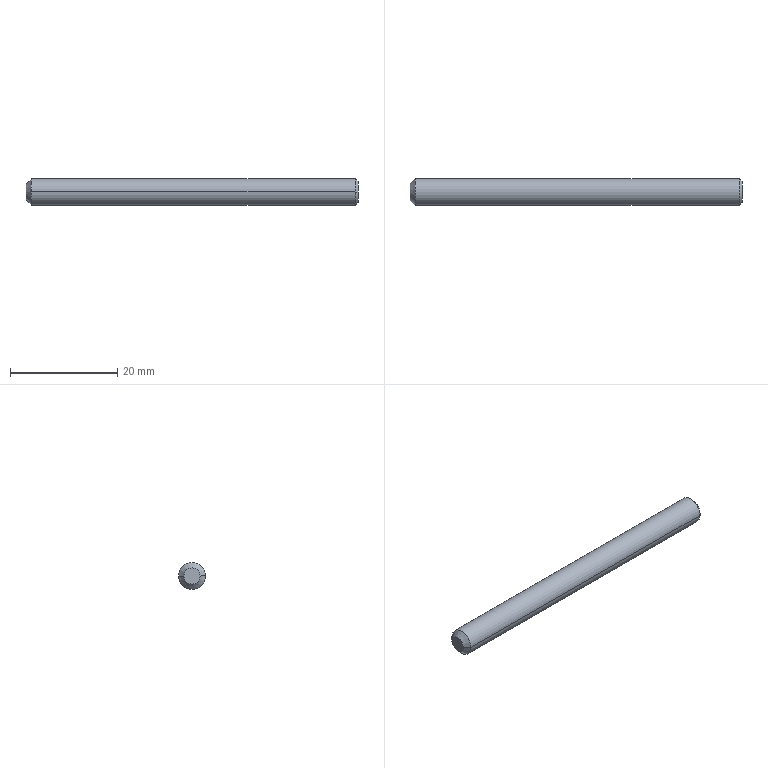Part | STEP file | ZHUANZHOU1_2_1_2_1_1 | 1 solid | 8 faces | box 62 x 5 x 5 mm | volume 1209 mm3 | cone 4 | plane 2 | cylinder 2 | commonest cylinder face diameters 5 x2
STEP:
#1=CARTESIAN_POINT('',(0.,0.,0.));
#2=DIRECTION('',(0.,0.,1.));
#3=DIRECTION('',(1.,0.,0.));
#4=AXIS2_PLACEMENT_3D('',#1,#2,#3);
#5=CARTESIAN_POINT('',(0.,-1.5,0.));
#6=VERTEX_POINT('',#5);
#7=CARTESIAN_POINT('',(0.,0.,-1.5));
#8=VERTEX_POINT('',#7);
#9=CARTESIAN_POINT('',(0.,0.,0.));
#10=DIRECTION('',(1.,0.,0.));
#11=DIRECTION('',(0.,-1.,0.));
#12=AXIS2_PLACEMENT_3D('',#9,#10,#11);
#13=CIRCLE('',#12,1.5);
#14=EDGE_CURVE('',#6,#8,#13,.T.);
#15=ORIENTED_EDGE('',*,*,#14,.T.);
#16=CARTESIAN_POINT('',(0.,1.5,0.));
#17=VERTEX_POINT('',#16);
#18=CARTESIAN_POINT('',(0.,0.,0.));
#19=DIRECTION('',(1.,0.,0.));
#20=DIRECTION('',(0.,0.,-1.));
#21=AXIS2_PLACEMENT_3D('',#18,#19,#20);
#22=CIRCLE('',#21,1.5);
#23=EDGE_CURVE('',#8,#17,#22,.T.);
#24=ORIENTED_EDGE('',*,*,#23,.T.);
#25=CARTESIAN_POINT('',(0.,0.,1.5));
#26=VERTEX_POINT('',#25);
#27=CARTESIAN_POINT('',(0.,0.,0.));
#28=DIRECTION('',(1.,0.,0.));
#29=DIRECTION('',(0.,1.,0.));
#30=AXIS2_PLACEMENT_3D('',#27,#28,#29);
#31=CIRCLE('',#30,1.5);
#32=EDGE_CURVE('',#17,#26,#31,.T.);
#33=ORIENTED_EDGE('',*,*,#32,.T.);
#34=CARTESIAN_POINT('',(0.,0.,0.));
#35=DIRECTION('',(1.,0.,0.));
#36=DIRECTION('',(0.,0.,1.));
#37=AXIS2_PLACEMENT_3D('',#34,#35,#36);
#38=CIRCLE('',#37,1.5);
#39=EDGE_CURVE('',#26,#6,#38,.T.);
#40=ORIENTED_EDGE('',*,*,#39,.T.);
#41=EDGE_LOOP('',(#15,#24,#33,#40));
#42=FACE_OUTER_BOUND('',#41,.F.);
#43=CARTESIAN_POINT('',(0.,0.,0.));
#44=DIRECTION('',(1.,0.,0.));
#45=DIRECTION('',(0.,-1.,0.));
#46=AXIS2_PLACEMENT_3D('',#43,#44,#45);
#47=PLANE('',#46);
#48=ADVANCED_FACE('',(#42),#47,.F.);
#49=ORIENTED_EDGE('',*,*,#23,.F.);
#50=ORIENTED_EDGE('',*,*,#14,.F.);
#51=CARTESIAN_POINT('',(1.,-2.5,0.));
#52=VERTEX_POINT('',#51);
#53=CARTESIAN_POINT('',(0.,-1.5,0.));
#54=DIRECTION('',(0.7071,-0.7071,0.));
#55=VECTOR('',#54,1.414);
#56=LINE('',#53,#55);
#57=EDGE_CURVE('',#6,#52,#56,.T.);
#58=ORIENTED_EDGE('',*,*,#57,.T.);
#59=CARTESIAN_POINT('',(1.,0.,-2.5));
#60=VERTEX_POINT('',#59);
#61=CARTESIAN_POINT('',(1.,0.,0.));
#62=DIRECTION('',(1.,0.,0.));
#63=DIRECTION('',(0.,-1.,0.));
#64=AXIS2_PLACEMENT_3D('',#61,#62,#63);
#65=CIRCLE('',#64,2.5);
#66=EDGE_CURVE('',#52,#60,#65,.T.);
#67=ORIENTED_EDGE('',*,*,#66,.T.);
#68=CARTESIAN_POINT('',(1.,2.5,-0.000000006));
#69=VERTEX_POINT('',#68);
#70=CARTESIAN_POINT('',(1.,0.,0.));
#71=DIRECTION('',(1.,0.,0.));
#72=DIRECTION('',(0.,0.,-1.));
#73=AXIS2_PLACEMENT_3D('',#70,#71,#72);
#74=CIRCLE('',#73,2.5);
#75=EDGE_CURVE('',#60,#69,#74,.T.);
#76=ORIENTED_EDGE('',*,*,#75,.T.);
#77=CARTESIAN_POINT('',(0.,1.5,-0.000000002));
#78=DIRECTION('',(0.7071,0.7071,-0.000000002));
#79=VECTOR('',#78,1.414);
#80=LINE('',#77,#79);
#81=EDGE_CURVE('',#17,#69,#80,.T.);
#82=ORIENTED_EDGE('',*,*,#81,.F.);
#83=EDGE_LOOP('',(#49,#50,#58,#67,#76,#82));
#84=FACE_OUTER_BOUND('',#83,.F.);
#85=CARTESIAN_POINT('',(0.5,0.,0.));
#86=DIRECTION('',(1.,0.,0.));
#87=DIRECTION('',(0.,0.,-1.));
#88=AXIS2_PLACEMENT_3D('',#85,#86,#87);
#89=CONICAL_SURFACE('',#88,2.,45.);
#90=ADVANCED_FACE('',(#84),#89,.T.);
#91=ORIENTED_EDGE('',*,*,#39,.F.);
#92=ORIENTED_EDGE('',*,*,#32,.F.);
#93=ORIENTED_EDGE('',*,*,#81,.T.);
#94=CARTESIAN_POINT('',(1.,0.,2.5));
#95=VERTEX_POINT('',#94);
#96=CARTESIAN_POINT('',(1.,0.,0.));
#97=DIRECTION('',(1.,0.,0.));
#98=DIRECTION('',(0.,1.,-0.000000002));
#99=AXIS2_PLACEMENT_3D('',#96,#97,#98);
#100=CIRCLE('',#99,2.5);
#101=EDGE_CURVE('',#69,#95,#100,.T.);
#102=ORIENTED_EDGE('',*,*,#101,.T.);
#103=CARTESIAN_POINT('',(1.,0.,0.));
#104=DIRECTION('',(1.,0.,0.));
#105=DIRECTION('',(0.,0.,1.));
#106=AXIS2_PLACEMENT_3D('',#103,#104,#105);
#107=CIRCLE('',#106,2.5);
#108=EDGE_CURVE('',#95,#52,#107,.T.);
#109=ORIENTED_EDGE('',*,*,#108,.T.);
#110=ORIENTED_EDGE('',*,*,#57,.F.);
#111=EDGE_LOOP('',(#91,#92,#93,#102,#109,#110));
#112=FACE_OUTER_BOUND('',#111,.F.);
#113=CARTESIAN_POINT('',(0.5,0.,0.));
#114=DIRECTION('',(1.,0.,0.));
#115=DIRECTION('',(0.,0.,-1.));
#116=AXIS2_PLACEMENT_3D('',#113,#114,#115);
#117=CONICAL_SURFACE('',#116,2.,45.);
#118=ADVANCED_FACE('',(#112),#117,.T.);
#119=CARTESIAN_POINT('',(61.5,0.,2.5));
#120=VERTEX_POINT('',#119);
#121=CARTESIAN_POINT('',(61.5,2.5,-0.000000006));
#122=VERTEX_POINT('',#121);
#123=CARTESIAN_POINT('',(61.5,0.,0.));
#124=DIRECTION('',(-1.,0.,0.));
#125=DIRECTION('',(0.,0.,1.));
#126=AXIS2_PLACEMENT_3D('',#123,#124,#125);
#127=CIRCLE('',#126,2.5);
#128=EDGE_CURVE('',#120,#122,#127,.T.);
#129=ORIENTED_EDGE('',*,*,#128,.F.);
#130=CARTESIAN_POINT('',(61.5,-2.5,0.));
#131=VERTEX_POINT('',#130);
#132=CARTESIAN_POINT('',(61.5,0.,0.));
#133=DIRECTION('',(-1.,0.,0.));
#134=DIRECTION('',(0.,-1.,0.));
#135=AXIS2_PLACEMENT_3D('',#132,#133,#134);
#136=CIRCLE('',#135,2.5);
#137=EDGE_CURVE('',#131,#120,#136,.T.);
#138=ORIENTED_EDGE('',*,*,#137,.F.);
#139=CARTESIAN_POINT('',(1.,-2.5,0.));
#140=DIRECTION('',(1.,0.,0.));
#141=VECTOR('',#140,60.5);
#142=LINE('',#139,#141);
#143=EDGE_CURVE('',#52,#131,#142,.T.);
#144=ORIENTED_EDGE('',*,*,#143,.F.);
#145=ORIENTED_EDGE('',*,*,#108,.F.);
#146=ORIENTED_EDGE('',*,*,#101,.F.);
#147=CARTESIAN_POINT('',(1.,2.5,-0.000000005));
#148=DIRECTION('',(1.,0.,0.));
#149=VECTOR('',#148,60.5);
#150=LINE('',#147,#149);
#151=EDGE_CURVE('',#69,#122,#150,.T.);
#152=ORIENTED_EDGE('',*,*,#151,.T.);
#153=EDGE_LOOP('',(#129,#138,#144,#145,#146,#152));
#154=FACE_OUTER_BOUND('',#153,.F.);
#155=CARTESIAN_POINT('',(0.,0.,0.));
#156=DIRECTION('',(1.,0.,0.));
#157=DIRECTION('',(0.,-1.,0.));
#158=AXIS2_PLACEMENT_3D('',#155,#156,#157);
#159=CYLINDRICAL_SURFACE('',#158,2.5);
#160=ADVANCED_FACE('',(#154),#159,.T.);
#161=CARTESIAN_POINT('',(62.,0.,2.));
#162=VERTEX_POINT('',#161);
#163=CARTESIAN_POINT('',(62.,2.,0.));
#164=VERTEX_POINT('',#163);
#165=CARTESIAN_POINT('',(62.,0.,0.));
#166=DIRECTION('',(-1.,0.,0.));
#167=DIRECTION('',(0.,0.,1.));
#168=AXIS2_PLACEMENT_3D('',#165,#166,#167);
#169=CIRCLE('',#168,2.);
#170=EDGE_CURVE('',#162,#164,#169,.T.);
#171=ORIENTED_EDGE('',*,*,#170,.F.);
#172=CARTESIAN_POINT('',(62.,-2.,0.));
#173=VERTEX_POINT('',#172);
#174=CARTESIAN_POINT('',(62.,0.,0.));
#175=DIRECTION('',(-1.,0.,0.));
#176=DIRECTION('',(0.,-1.,0.));
#177=AXIS2_PLACEMENT_3D('',#174,#175,#176);
#178=CIRCLE('',#177,2.);
#179=EDGE_CURVE('',#173,#162,#178,.T.);
#180=ORIENTED_EDGE('',*,*,#179,.F.);
#181=CARTESIAN_POINT('',(62.,-2.,0.000000001));
#182=DIRECTION('',(-0.7071,-0.7071,0.));
#183=VECTOR('',#182,0.7071);
#184=LINE('',#181,#183);
#185=EDGE_CURVE('',#173,#131,#184,.T.);
#186=ORIENTED_EDGE('',*,*,#185,.T.);
#187=ORIENTED_EDGE('',*,*,#137,.T.);
#188=ORIENTED_EDGE('',*,*,#128,.T.);
#189=CARTESIAN_POINT('',(62.,2.,-0.000000003));
#190=DIRECTION('',(-0.7071,0.7071,-0.000000004));
#191=VECTOR('',#190,0.7071);
#192=LINE('',#189,#191);
#193=EDGE_CURVE('',#164,#122,#192,.T.);
#194=ORIENTED_EDGE('',*,*,#193,.F.);
#195=EDGE_LOOP('',(#171,#180,#186,#187,#188,#194));
#196=FACE_OUTER_BOUND('',#195,.F.);
#197=CARTESIAN_POINT('',(61.75,0.,0.));
#198=DIRECTION('',(-1.,0.,0.));
#199=DIRECTION('',(0.,0.,-1.));
#200=AXIS2_PLACEMENT_3D('',#197,#198,#199);
#201=CONICAL_SURFACE('',#200,2.25,45.);
#202=ADVANCED_FACE('',(#196),#201,.T.);
#203=CARTESIAN_POINT('',(62.,0.,-2.));
#204=VERTEX_POINT('',#203);
#205=CARTESIAN_POINT('',(62.,0.,0.));
#206=DIRECTION('',(-1.,0.,0.));
#207=DIRECTION('',(0.,1.,0.));
#208=AXIS2_PLACEMENT_3D('',#205,#206,#207);
#209=CIRCLE('',#208,2.);
#210=EDGE_CURVE('',#164,#204,#209,.T.);
#211=ORIENTED_EDGE('',*,*,#210,.T.);
#212=CARTESIAN_POINT('',(62.,0.,0.));
#213=DIRECTION('',(-1.,0.,0.));
#214=DIRECTION('',(0.,0.,-1.));
#215=AXIS2_PLACEMENT_3D('',#212,#213,#214);
#216=CIRCLE('',#215,2.);
#217=EDGE_CURVE('',#204,#173,#216,.T.);
#218=ORIENTED_EDGE('',*,*,#217,.T.);
#219=ORIENTED_EDGE('',*,*,#179,.T.);
#220=ORIENTED_EDGE('',*,*,#170,.T.);
#221=EDGE_LOOP('',(#211,#218,#219,#220));
#222=FACE_OUTER_BOUND('',#221,.F.);
#223=CARTESIAN_POINT('',(62.,0.,0.));
#224=DIRECTION('',(1.,0.,0.));
#225=DIRECTION('',(0.,-1.,0.));
#226=AXIS2_PLACEMENT_3D('',#223,#224,#225);
#227=PLANE('',#226);
#228=ADVANCED_FACE('',(#222),#227,.T.);
#229=ORIENTED_EDGE('',*,*,#217,.F.);
#230=ORIENTED_EDGE('',*,*,#210,.F.);
#231=ORIENTED_EDGE('',*,*,#193,.T.);
#232=CARTESIAN_POINT('',(61.5,0.,-2.5));
#233=VERTEX_POINT('',#232);
#234=CARTESIAN_POINT('',(61.5,0.,0.));
#235=DIRECTION('',(-1.,0.,0.));
#236=DIRECTION('',(0.,1.,-0.000000002));
#237=AXIS2_PLACEMENT_3D('',#234,#235,#236);
#238=CIRCLE('',#237,2.5);
#239=EDGE_CURVE('',#122,#233,#238,.T.);
#240=ORIENTED_EDGE('',*,*,#239,.T.);
#241=CARTESIAN_POINT('',(61.5,0.,0.));
#242=DIRECTION('',(-1.,0.,0.));
#243=DIRECTION('',(0.,0.,-1.));
#244=AXIS2_PLACEMENT_3D('',#241,#242,#243);
#245=CIRCLE('',#244,2.5);
#246=EDGE_CURVE('',#233,#131,#245,.T.);
#247=ORIENTED_EDGE('',*,*,#246,.T.);
#248=ORIENTED_EDGE('',*,*,#185,.F.);
#249=EDGE_LOOP('',(#229,#230,#231,#240,#247,#248));
#250=FACE_OUTER_BOUND('',#249,.F.);
#251=CARTESIAN_POINT('',(61.75,0.,0.));
#252=DIRECTION('',(-1.,0.,0.));
#253=DIRECTION('',(0.,0.,-1.));
#254=AXIS2_PLACEMENT_3D('',#251,#252,#253);
#255=CONICAL_SURFACE('',#254,2.25,45.);
#256=ADVANCED_FACE('',(#250),#255,.T.);
#257=ORIENTED_EDGE('',*,*,#246,.F.);
#258=ORIENTED_EDGE('',*,*,#239,.F.);
#259=ORIENTED_EDGE('',*,*,#151,.F.);
#260=ORIENTED_EDGE('',*,*,#75,.F.);
#261=ORIENTED_EDGE('',*,*,#66,.F.);
#262=ORIENTED_EDGE('',*,*,#143,.T.);
#263=EDGE_LOOP('',(#257,#258,#259,#260,#261,#262));
#264=FACE_OUTER_BOUND('',#263,.F.);
#265=CARTESIAN_POINT('',(0.,0.,0.));
#266=DIRECTION('',(1.,0.,0.));
#267=DIRECTION('',(0.,-1.,0.));
#268=AXIS2_PLACEMENT_3D('',#265,#266,#267);
#269=CYLINDRICAL_SURFACE('',#268,2.5);
#270=ADVANCED_FACE('',(#264),#269,.T.);
#271=CLOSED_SHELL('',(#48,#90,#118,#160,#202,#228,#256,#270));
#272=MANIFOLD_SOLID_BREP('',#271);
#273=(LENGTH_UNIT()NAMED_UNIT(*)SI_UNIT(.MILLI.,.METRE.));
#274=UNCERTAINTY_MEASURE_WITH_UNIT(LENGTH_MEASURE(0.00624),#273,'','');
#275=(NAMED_UNIT(*)PLANE_ANGLE_UNIT()SI_UNIT($,.RADIAN.));
#276=PLANE_ANGLE_MEASURE_WITH_UNIT(PLANE_ANGLE_MEASURE(0.01745),#275);
#277=(CONVERSION_BASED_UNIT('DEGREE',#276)NAMED_UNIT(*)PLANE_ANGLE_UNIT());
#278=(NAMED_UNIT(*)SI_UNIT($,.STERADIAN.)SOLID_ANGLE_UNIT());
#279=(GEOMETRIC_REPRESENTATION_CONTEXT(3)GLOBAL_UNCERTAINTY_ASSIGNED_CONTEXT((#274))GLOBAL_UNIT_ASSIGNED_CONTEXT((#273,#277,#278))REPRESENTATION_CONTEXT('',''));
#280=ADVANCED_BREP_SHAPE_REPRESENTATION('',(#4,#272),#279);